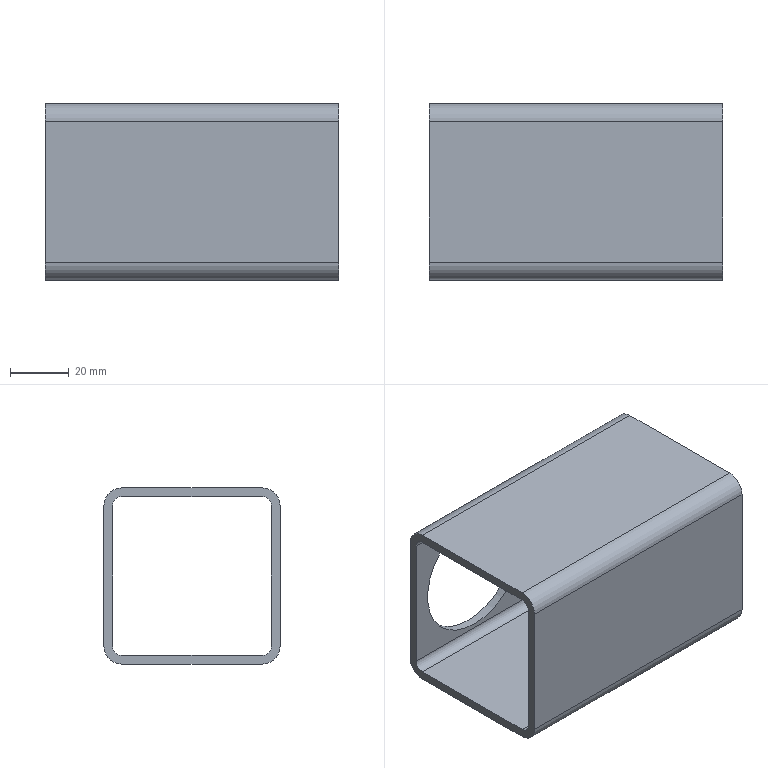Part | STEP file | JBJ-P-1013-03_Default<As Machined> | 1 solid | 19 faces | box 100 x 60 x 60 mm | volume 61311 mm3 | plane 10 | cylinder 9 | commonest cylinder face diameters 6 x4 12 x4 45 x1
STEP:
#1=CARTESIAN_POINT('',(0.,-30.,24.));
#2=VERTEX_POINT('',#1);
#3=CARTESIAN_POINT('',(0.,-24.,30.));
#4=VERTEX_POINT('',#3);
#5=CARTESIAN_POINT('',(0.,-24.,24.));
#6=DIRECTION('',(-1.,0.,0.));
#7=DIRECTION('',(0.,0.,1.));
#8=AXIS2_PLACEMENT_3D('',#5,#6,#7);
#9=CIRCLE('',#8,6.);
#10=EDGE_CURVE('',#2,#4,#9,.T.);
#11=ORIENTED_EDGE('',*,*,#10,.T.);
#12=CARTESIAN_POINT('',(-100.,-24.,30.));
#13=VERTEX_POINT('',#12);
#14=CARTESIAN_POINT('',(-100.,-24.,30.));
#15=DIRECTION('',(1.,0.,0.));
#16=VECTOR('',#15,1000.);
#17=LINE('',#14,#16);
#18=EDGE_CURVE('',#13,#4,#17,.T.);
#19=ORIENTED_EDGE('',*,*,#18,.F.);
#20=CARTESIAN_POINT('',(-100.,-30.,24.));
#21=VERTEX_POINT('',#20);
#22=CARTESIAN_POINT('',(-100.,-24.,24.));
#23=DIRECTION('',(-1.,0.,0.));
#24=DIRECTION('',(0.,0.,1.));
#25=AXIS2_PLACEMENT_3D('',#22,#23,#24);
#26=CIRCLE('',#25,6.);
#27=EDGE_CURVE('',#21,#13,#26,.T.);
#28=ORIENTED_EDGE('',*,*,#27,.F.);
#29=CARTESIAN_POINT('',(-100.,-30.,24.));
#30=DIRECTION('',(1.,0.,0.));
#31=VECTOR('',#30,1000.);
#32=LINE('',#29,#31);
#33=EDGE_CURVE('',#21,#2,#32,.T.);
#34=ORIENTED_EDGE('',*,*,#33,.T.);
#35=EDGE_LOOP('',(#11,#19,#28,#34));
#36=FACE_OUTER_BOUND('',#35,.T.);
#37=CARTESIAN_POINT('',(-100.,-24.,24.));
#38=DIRECTION('',(1.,0.,0.));
#39=DIRECTION('',(0.,0.,-1.));
#40=AXIS2_PLACEMENT_3D('',#37,#38,#39);
#41=CYLINDRICAL_SURFACE('',#40,6.);
#42=ADVANCED_FACE('',(#36),#41,.T.);
#43=CARTESIAN_POINT('',(0.,24.,30.));
#44=VERTEX_POINT('',#43);
#45=CARTESIAN_POINT('',(0.,-24.,30.));
#46=DIRECTION('',(0.,1.,0.));
#47=VECTOR('',#46,1000.);
#48=LINE('',#45,#47);
#49=EDGE_CURVE('',#4,#44,#48,.T.);
#50=ORIENTED_EDGE('',*,*,#49,.T.);
#51=CARTESIAN_POINT('',(-100.,24.,30.));
#52=VERTEX_POINT('',#51);
#53=CARTESIAN_POINT('',(-100.,24.,30.));
#54=DIRECTION('',(1.,0.,0.));
#55=VECTOR('',#54,1000.);
#56=LINE('',#53,#55);
#57=EDGE_CURVE('',#52,#44,#56,.T.);
#58=ORIENTED_EDGE('',*,*,#57,.F.);
#59=CARTESIAN_POINT('',(-100.,-24.,30.));
#60=DIRECTION('',(0.,1.,0.));
#61=VECTOR('',#60,1000.);
#62=LINE('',#59,#61);
#63=EDGE_CURVE('',#13,#52,#62,.T.);
#64=ORIENTED_EDGE('',*,*,#63,.F.);
#65=ORIENTED_EDGE('',*,*,#18,.T.);
#66=EDGE_LOOP('',(#50,#58,#64,#65));
#67=FACE_OUTER_BOUND('',#66,.T.);
#68=CARTESIAN_POINT('',(-100.,-24.,30.));
#69=DIRECTION('',(0.,0.,-1.));
#70=DIRECTION('',(-1.,0.,0.));
#71=AXIS2_PLACEMENT_3D('',#68,#69,#70);
#72=PLANE('',#71);
#73=ADVANCED_FACE('',(#67),#72,.F.);
#74=CARTESIAN_POINT('',(0.,30.,24.));
#75=VERTEX_POINT('',#74);
#76=CARTESIAN_POINT('',(0.,24.,24.));
#77=DIRECTION('',(-1.,0.,0.));
#78=DIRECTION('',(0.,0.,1.));
#79=AXIS2_PLACEMENT_3D('',#76,#77,#78);
#80=CIRCLE('',#79,6.);
#81=EDGE_CURVE('',#44,#75,#80,.T.);
#82=ORIENTED_EDGE('',*,*,#81,.T.);
#83=CARTESIAN_POINT('',(-100.,30.,24.));
#84=VERTEX_POINT('',#83);
#85=CARTESIAN_POINT('',(-100.,30.,24.));
#86=DIRECTION('',(1.,0.,0.));
#87=VECTOR('',#86,1000.);
#88=LINE('',#85,#87);
#89=EDGE_CURVE('',#84,#75,#88,.T.);
#90=ORIENTED_EDGE('',*,*,#89,.F.);
#91=CARTESIAN_POINT('',(-100.,24.,24.));
#92=DIRECTION('',(-1.,0.,0.));
#93=DIRECTION('',(0.,0.,1.));
#94=AXIS2_PLACEMENT_3D('',#91,#92,#93);
#95=CIRCLE('',#94,6.);
#96=EDGE_CURVE('',#52,#84,#95,.T.);
#97=ORIENTED_EDGE('',*,*,#96,.F.);
#98=ORIENTED_EDGE('',*,*,#57,.T.);
#99=EDGE_LOOP('',(#82,#90,#97,#98));
#100=FACE_OUTER_BOUND('',#99,.T.);
#101=CARTESIAN_POINT('',(-100.,24.,24.));
#102=DIRECTION('',(1.,0.,0.));
#103=DIRECTION('',(0.,0.,-1.));
#104=AXIS2_PLACEMENT_3D('',#101,#102,#103);
#105=CYLINDRICAL_SURFACE('',#104,6.);
#106=ADVANCED_FACE('',(#100),#105,.T.);
#107=CARTESIAN_POINT('',(-72.,30.,22.5));
#108=VERTEX_POINT('',#107);
#109=CARTESIAN_POINT('',(-72.,30.,0.));
#110=DIRECTION('',(0.,1.,0.));
#111=DIRECTION('',(0.,0.,1.));
#112=AXIS2_PLACEMENT_3D('',#109,#110,#111);
#113=CIRCLE('',#112,22.5);
#114=EDGE_CURVE('',#108,#108,#113,.T.);
#115=ORIENTED_EDGE('',*,*,#114,.F.);
#116=EDGE_LOOP('',(#115));
#117=FACE_BOUND('',#116,.T.);
#118=CARTESIAN_POINT('',(0.,30.,-24.));
#119=VERTEX_POINT('',#118);
#120=CARTESIAN_POINT('',(0.,30.,-24.));
#121=DIRECTION('',(0.,0.,-1.));
#122=VECTOR('',#121,1000.);
#123=LINE('',#120,#122);
#124=EDGE_CURVE('',#75,#119,#123,.T.);
#125=ORIENTED_EDGE('',*,*,#124,.T.);
#126=CARTESIAN_POINT('',(-100.,30.,-24.));
#127=VERTEX_POINT('',#126);
#128=CARTESIAN_POINT('',(-100.,30.,-24.));
#129=DIRECTION('',(1.,0.,0.));
#130=VECTOR('',#129,1000.);
#131=LINE('',#128,#130);
#132=EDGE_CURVE('',#127,#119,#131,.T.);
#133=ORIENTED_EDGE('',*,*,#132,.F.);
#134=CARTESIAN_POINT('',(-100.,30.,-24.));
#135=DIRECTION('',(0.,0.,-1.));
#136=VECTOR('',#135,1000.);
#137=LINE('',#134,#136);
#138=EDGE_CURVE('',#84,#127,#137,.T.);
#139=ORIENTED_EDGE('',*,*,#138,.F.);
#140=ORIENTED_EDGE('',*,*,#89,.T.);
#141=EDGE_LOOP('',(#125,#133,#139,#140));
#142=FACE_OUTER_BOUND('',#141,.T.);
#143=CARTESIAN_POINT('',(-100.,30.,-24.));
#144=DIRECTION('',(0.,-1.,0.));
#145=DIRECTION('',(0.,0.,-1.));
#146=AXIS2_PLACEMENT_3D('',#143,#144,#145);
#147=PLANE('',#146);
#148=ADVANCED_FACE('',(#117,#142),#147,.F.);
#149=CARTESIAN_POINT('',(0.,24.,-30.));
#150=VERTEX_POINT('',#149);
#151=CARTESIAN_POINT('',(0.,24.,-24.));
#152=DIRECTION('',(-1.,0.,0.));
#153=DIRECTION('',(0.,0.,1.));
#154=AXIS2_PLACEMENT_3D('',#151,#152,#153);
#155=CIRCLE('',#154,6.);
#156=EDGE_CURVE('',#119,#150,#155,.T.);
#157=ORIENTED_EDGE('',*,*,#156,.T.);
#158=CARTESIAN_POINT('',(-100.,24.,-30.));
#159=VERTEX_POINT('',#158);
#160=CARTESIAN_POINT('',(-100.,24.,-30.));
#161=DIRECTION('',(1.,0.,0.));
#162=VECTOR('',#161,1000.);
#163=LINE('',#160,#162);
#164=EDGE_CURVE('',#159,#150,#163,.T.);
#165=ORIENTED_EDGE('',*,*,#164,.F.);
#166=CARTESIAN_POINT('',(-100.,24.,-24.));
#167=DIRECTION('',(-1.,0.,0.));
#168=DIRECTION('',(0.,0.,1.));
#169=AXIS2_PLACEMENT_3D('',#166,#167,#168);
#170=CIRCLE('',#169,6.);
#171=EDGE_CURVE('',#127,#159,#170,.T.);
#172=ORIENTED_EDGE('',*,*,#171,.F.);
#173=ORIENTED_EDGE('',*,*,#132,.T.);
#174=EDGE_LOOP('',(#157,#165,#172,#173));
#175=FACE_OUTER_BOUND('',#174,.T.);
#176=CARTESIAN_POINT('',(-100.,24.,-24.));
#177=DIRECTION('',(1.,0.,0.));
#178=DIRECTION('',(0.,0.,-1.));
#179=AXIS2_PLACEMENT_3D('',#176,#177,#178);
#180=CYLINDRICAL_SURFACE('',#179,6.);
#181=ADVANCED_FACE('',(#175),#180,.T.);
#182=CARTESIAN_POINT('',(0.,-24.,-30.));
#183=VERTEX_POINT('',#182);
#184=CARTESIAN_POINT('',(0.,24.,-30.));
#185=DIRECTION('',(0.,-1.,0.));
#186=VECTOR('',#185,1000.);
#187=LINE('',#184,#186);
#188=EDGE_CURVE('',#150,#183,#187,.T.);
#189=ORIENTED_EDGE('',*,*,#188,.T.);
#190=CARTESIAN_POINT('',(-100.,-24.,-30.));
#191=VERTEX_POINT('',#190);
#192=CARTESIAN_POINT('',(-100.,-24.,-30.));
#193=DIRECTION('',(1.,0.,0.));
#194=VECTOR('',#193,1000.);
#195=LINE('',#192,#194);
#196=EDGE_CURVE('',#191,#183,#195,.T.);
#197=ORIENTED_EDGE('',*,*,#196,.F.);
#198=CARTESIAN_POINT('',(-100.,24.,-30.));
#199=DIRECTION('',(0.,-1.,0.));
#200=VECTOR('',#199,1000.);
#201=LINE('',#198,#200);
#202=EDGE_CURVE('',#159,#191,#201,.T.);
#203=ORIENTED_EDGE('',*,*,#202,.F.);
#204=ORIENTED_EDGE('',*,*,#164,.T.);
#205=EDGE_LOOP('',(#189,#197,#203,#204));
#206=FACE_OUTER_BOUND('',#205,.T.);
#207=CARTESIAN_POINT('',(-100.,24.,-30.));
#208=DIRECTION('',(0.,0.,1.));
#209=DIRECTION('',(1.,0.,0.));
#210=AXIS2_PLACEMENT_3D('',#207,#208,#209);
#211=PLANE('',#210);
#212=ADVANCED_FACE('',(#206),#211,.F.);
#213=CARTESIAN_POINT('',(0.,-30.,-24.));
#214=VERTEX_POINT('',#213);
#215=CARTESIAN_POINT('',(0.,-24.,-24.));
#216=DIRECTION('',(-1.,0.,0.));
#217=DIRECTION('',(0.,0.,1.));
#218=AXIS2_PLACEMENT_3D('',#215,#216,#217);
#219=CIRCLE('',#218,6.);
#220=EDGE_CURVE('',#183,#214,#219,.T.);
#221=ORIENTED_EDGE('',*,*,#220,.T.);
#222=CARTESIAN_POINT('',(-100.,-30.,-24.));
#223=VERTEX_POINT('',#222);
#224=CARTESIAN_POINT('',(-100.,-30.,-24.));
#225=DIRECTION('',(1.,0.,0.));
#226=VECTOR('',#225,1000.);
#227=LINE('',#224,#226);
#228=EDGE_CURVE('',#223,#214,#227,.T.);
#229=ORIENTED_EDGE('',*,*,#228,.F.);
#230=CARTESIAN_POINT('',(-100.,-24.,-24.));
#231=DIRECTION('',(-1.,0.,0.));
#232=DIRECTION('',(0.,0.,1.));
#233=AXIS2_PLACEMENT_3D('',#230,#231,#232);
#234=CIRCLE('',#233,6.);
#235=EDGE_CURVE('',#191,#223,#234,.T.);
#236=ORIENTED_EDGE('',*,*,#235,.F.);
#237=ORIENTED_EDGE('',*,*,#196,.T.);
#238=EDGE_LOOP('',(#221,#229,#236,#237));
#239=FACE_OUTER_BOUND('',#238,.T.);
#240=CARTESIAN_POINT('',(-100.,-24.,-24.));
#241=DIRECTION('',(1.,0.,0.));
#242=DIRECTION('',(0.,0.,-1.));
#243=AXIS2_PLACEMENT_3D('',#240,#241,#242);
#244=CYLINDRICAL_SURFACE('',#243,6.);
#245=ADVANCED_FACE('',(#239),#244,.T.);
#246=CARTESIAN_POINT('',(0.,24.,27.));
#247=VERTEX_POINT('',#246);
#248=CARTESIAN_POINT('',(0.,27.,24.));
#249=VERTEX_POINT('',#248);
#250=CARTESIAN_POINT('',(0.,24.,24.));
#251=DIRECTION('',(-1.,0.,0.));
#252=DIRECTION('',(0.,0.,1.));
#253=AXIS2_PLACEMENT_3D('',#250,#251,#252);
#254=CIRCLE('',#253,3.);
#255=EDGE_CURVE('',#247,#249,#254,.T.);
#256=ORIENTED_EDGE('',*,*,#255,.F.);
#257=CARTESIAN_POINT('',(-100.,24.,27.));
#258=VERTEX_POINT('',#257);
#259=CARTESIAN_POINT('',(-100.,24.,27.));
#260=DIRECTION('',(1.,0.,0.));
#261=VECTOR('',#260,1000.);
#262=LINE('',#259,#261);
#263=EDGE_CURVE('',#258,#247,#262,.T.);
#264=ORIENTED_EDGE('',*,*,#263,.F.);
#265=CARTESIAN_POINT('',(-100.,27.,24.));
#266=VERTEX_POINT('',#265);
#267=CARTESIAN_POINT('',(-100.,24.,24.));
#268=DIRECTION('',(-1.,0.,0.));
#269=DIRECTION('',(0.,0.,1.));
#270=AXIS2_PLACEMENT_3D('',#267,#268,#269);
#271=CIRCLE('',#270,3.);
#272=EDGE_CURVE('',#258,#266,#271,.T.);
#273=ORIENTED_EDGE('',*,*,#272,.T.);
#274=CARTESIAN_POINT('',(-100.,27.,24.));
#275=DIRECTION('',(1.,0.,0.));
#276=VECTOR('',#275,1000.);
#277=LINE('',#274,#276);
#278=EDGE_CURVE('',#266,#249,#277,.T.);
#279=ORIENTED_EDGE('',*,*,#278,.T.);
#280=EDGE_LOOP('',(#256,#264,#273,#279));
#281=FACE_OUTER_BOUND('',#280,.T.);
#282=CARTESIAN_POINT('',(-100.,24.,24.));
#283=DIRECTION('',(1.,0.,0.));
#284=DIRECTION('',(0.,0.,-1.));
#285=AXIS2_PLACEMENT_3D('',#282,#283,#284);
#286=CYLINDRICAL_SURFACE('',#285,3.);
#287=ADVANCED_FACE('',(#281),#286,.F.);
#288=CARTESIAN_POINT('',(0.,-24.,27.));
#289=VERTEX_POINT('',#288);
#290=CARTESIAN_POINT('',(0.,-24.,27.));
#291=DIRECTION('',(0.,1.,0.));
#292=VECTOR('',#291,1000.);
#293=LINE('',#290,#292);
#294=EDGE_CURVE('',#289,#247,#293,.T.);
#295=ORIENTED_EDGE('',*,*,#294,.F.);
#296=CARTESIAN_POINT('',(-100.,-24.,27.));
#297=VERTEX_POINT('',#296);
#298=CARTESIAN_POINT('',(-100.,-24.,27.));
#299=DIRECTION('',(1.,0.,0.));
#300=VECTOR('',#299,1000.);
#301=LINE('',#298,#300);
#302=EDGE_CURVE('',#297,#289,#301,.T.);
#303=ORIENTED_EDGE('',*,*,#302,.F.);
#304=CARTESIAN_POINT('',(-100.,-24.,27.));
#305=DIRECTION('',(0.,1.,0.));
#306=VECTOR('',#305,1000.);
#307=LINE('',#304,#306);
#308=EDGE_CURVE('',#297,#258,#307,.T.);
#309=ORIENTED_EDGE('',*,*,#308,.T.);
#310=ORIENTED_EDGE('',*,*,#263,.T.);
#311=EDGE_LOOP('',(#295,#303,#309,#310));
#312=FACE_OUTER_BOUND('',#311,.T.);
#313=CARTESIAN_POINT('',(-100.,-24.,27.));
#314=DIRECTION('',(0.,0.,-1.));
#315=DIRECTION('',(-1.,0.,0.));
#316=AXIS2_PLACEMENT_3D('',#313,#314,#315);
#317=PLANE('',#316);
#318=ADVANCED_FACE('',(#312),#317,.T.);
#319=CARTESIAN_POINT('',(0.,-27.,24.));
#320=VERTEX_POINT('',#319);
#321=CARTESIAN_POINT('',(0.,-24.,24.));
#322=DIRECTION('',(-1.,0.,0.));
#323=DIRECTION('',(0.,0.,1.));
#324=AXIS2_PLACEMENT_3D('',#321,#322,#323);
#325=CIRCLE('',#324,3.);
#326=EDGE_CURVE('',#320,#289,#325,.T.);
#327=ORIENTED_EDGE('',*,*,#326,.F.);
#328=CARTESIAN_POINT('',(-100.,-27.,24.));
#329=VERTEX_POINT('',#328);
#330=CARTESIAN_POINT('',(-100.,-27.,24.));
#331=DIRECTION('',(1.,0.,0.));
#332=VECTOR('',#331,1000.);
#333=LINE('',#330,#332);
#334=EDGE_CURVE('',#329,#320,#333,.T.);
#335=ORIENTED_EDGE('',*,*,#334,.F.);
#336=CARTESIAN_POINT('',(-100.,-24.,24.));
#337=DIRECTION('',(-1.,0.,0.));
#338=DIRECTION('',(0.,0.,1.));
#339=AXIS2_PLACEMENT_3D('',#336,#337,#338);
#340=CIRCLE('',#339,3.);
#341=EDGE_CURVE('',#329,#297,#340,.T.);
#342=ORIENTED_EDGE('',*,*,#341,.T.);
#343=ORIENTED_EDGE('',*,*,#302,.T.);
#344=EDGE_LOOP('',(#327,#335,#342,#343));
#345=FACE_OUTER_BOUND('',#344,.T.);
#346=CARTESIAN_POINT('',(-100.,-24.,24.));
#347=DIRECTION('',(1.,0.,0.));
#348=DIRECTION('',(0.,0.,-1.));
#349=AXIS2_PLACEMENT_3D('',#346,#347,#348);
#350=CYLINDRICAL_SURFACE('',#349,3.);
#351=ADVANCED_FACE('',(#345),#350,.F.);
#352=CARTESIAN_POINT('',(0.,-27.,-24.));
#353=VERTEX_POINT('',#352);
#354=CARTESIAN_POINT('',(0.,-27.,24.));
#355=DIRECTION('',(0.,0.,1.));
#356=VECTOR('',#355,1000.);
#357=LINE('',#354,#356);
#358=EDGE_CURVE('',#353,#320,#357,.T.);
#359=ORIENTED_EDGE('',*,*,#358,.F.);
#360=CARTESIAN_POINT('',(-100.,-27.,-24.));
#361=VERTEX_POINT('',#360);
#362=CARTESIAN_POINT('',(-100.,-27.,-24.));
#363=DIRECTION('',(1.,0.,0.));
#364=VECTOR('',#363,1000.);
#365=LINE('',#362,#364);
#366=EDGE_CURVE('',#361,#353,#365,.T.);
#367=ORIENTED_EDGE('',*,*,#366,.F.);
#368=CARTESIAN_POINT('',(-100.,-27.,24.));
#369=DIRECTION('',(0.,0.,1.));
#370=VECTOR('',#369,1000.);
#371=LINE('',#368,#370);
#372=EDGE_CURVE('',#361,#329,#371,.T.);
#373=ORIENTED_EDGE('',*,*,#372,.T.);
#374=ORIENTED_EDGE('',*,*,#334,.T.);
#375=EDGE_LOOP('',(#359,#367,#373,#374));
#376=FACE_OUTER_BOUND('',#375,.T.);
#377=CARTESIAN_POINT('',(-100.,-27.,24.));
#378=DIRECTION('',(0.,1.,0.));
#379=DIRECTION('',(0.,0.,1.));
#380=AXIS2_PLACEMENT_3D('',#377,#378,#379);
#381=PLANE('',#380);
#382=ADVANCED_FACE('',(#376),#381,.T.);
#383=CARTESIAN_POINT('',(0.,-24.,-27.));
#384=VERTEX_POINT('',#383);
#385=CARTESIAN_POINT('',(0.,-24.,-24.));
#386=DIRECTION('',(-1.,0.,0.));
#387=DIRECTION('',(0.,0.,1.));
#388=AXIS2_PLACEMENT_3D('',#385,#386,#387);
#389=CIRCLE('',#388,3.);
#390=EDGE_CURVE('',#384,#353,#389,.T.);
#391=ORIENTED_EDGE('',*,*,#390,.F.);
#392=CARTESIAN_POINT('',(-100.,-24.,-27.));
#393=VERTEX_POINT('',#392);
#394=CARTESIAN_POINT('',(-100.,-24.,-27.));
#395=DIRECTION('',(1.,0.,0.));
#396=VECTOR('',#395,1000.);
#397=LINE('',#394,#396);
#398=EDGE_CURVE('',#393,#384,#397,.T.);
#399=ORIENTED_EDGE('',*,*,#398,.F.);
#400=CARTESIAN_POINT('',(-100.,-24.,-24.));
#401=DIRECTION('',(-1.,0.,0.));
#402=DIRECTION('',(0.,0.,1.));
#403=AXIS2_PLACEMENT_3D('',#400,#401,#402);
#404=CIRCLE('',#403,3.);
#405=EDGE_CURVE('',#393,#361,#404,.T.);
#406=ORIENTED_EDGE('',*,*,#405,.T.);
#407=ORIENTED_EDGE('',*,*,#366,.T.);
#408=EDGE_LOOP('',(#391,#399,#406,#407));
#409=FACE_OUTER_BOUND('',#408,.T.);
#410=CARTESIAN_POINT('',(-100.,-24.,-24.));
#411=DIRECTION('',(1.,0.,0.));
#412=DIRECTION('',(0.,0.,-1.));
#413=AXIS2_PLACEMENT_3D('',#410,#411,#412);
#414=CYLINDRICAL_SURFACE('',#413,3.);
#415=ADVANCED_FACE('',(#409),#414,.F.);
#416=CARTESIAN_POINT('',(0.,24.,-27.));
#417=VERTEX_POINT('',#416);
#418=CARTESIAN_POINT('',(0.,24.,-27.));
#419=DIRECTION('',(0.,-1.,0.));
#420=VECTOR('',#419,1000.);
#421=LINE('',#418,#420);
#422=EDGE_CURVE('',#417,#384,#421,.T.);
#423=ORIENTED_EDGE('',*,*,#422,.F.);
#424=CARTESIAN_POINT('',(-100.,24.,-27.));
#425=VERTEX_POINT('',#424);
#426=CARTESIAN_POINT('',(-100.,24.,-27.));
#427=DIRECTION('',(1.,0.,0.));
#428=VECTOR('',#427,1000.);
#429=LINE('',#426,#428);
#430=EDGE_CURVE('',#425,#417,#429,.T.);
#431=ORIENTED_EDGE('',*,*,#430,.F.);
#432=CARTESIAN_POINT('',(-100.,24.,-27.));
#433=DIRECTION('',(0.,-1.,0.));
#434=VECTOR('',#433,1000.);
#435=LINE('',#432,#434);
#436=EDGE_CURVE('',#425,#393,#435,.T.);
#437=ORIENTED_EDGE('',*,*,#436,.T.);
#438=ORIENTED_EDGE('',*,*,#398,.T.);
#439=EDGE_LOOP('',(#423,#431,#437,#438));
#440=FACE_OUTER_BOUND('',#439,.T.);
#441=CARTESIAN_POINT('',(-100.,24.,-27.));
#442=DIRECTION('',(0.,0.,1.));
#443=DIRECTION('',(1.,0.,0.));
#444=AXIS2_PLACEMENT_3D('',#441,#442,#443);
#445=PLANE('',#444);
#446=ADVANCED_FACE('',(#440),#445,.T.);
#447=CARTESIAN_POINT('',(0.,27.,-24.));
#448=VERTEX_POINT('',#447);
#449=CARTESIAN_POINT('',(0.,24.,-24.));
#450=DIRECTION('',(-1.,0.,0.));
#451=DIRECTION('',(0.,0.,1.));
#452=AXIS2_PLACEMENT_3D('',#449,#450,#451);
#453=CIRCLE('',#452,3.);
#454=EDGE_CURVE('',#448,#417,#453,.T.);
#455=ORIENTED_EDGE('',*,*,#454,.F.);
#456=CARTESIAN_POINT('',(-100.,27.,-24.));
#457=VERTEX_POINT('',#456);
#458=CARTESIAN_POINT('',(-100.,27.,-24.));
#459=DIRECTION('',(1.,0.,0.));
#460=VECTOR('',#459,1000.);
#461=LINE('',#458,#460);
#462=EDGE_CURVE('',#457,#448,#461,.T.);
#463=ORIENTED_EDGE('',*,*,#462,.F.);
#464=CARTESIAN_POINT('',(-100.,24.,-24.));
#465=DIRECTION('',(-1.,0.,0.));
#466=DIRECTION('',(0.,0.,1.));
#467=AXIS2_PLACEMENT_3D('',#464,#465,#466);
#468=CIRCLE('',#467,3.);
#469=EDGE_CURVE('',#457,#425,#468,.T.);
#470=ORIENTED_EDGE('',*,*,#469,.T.);
#471=ORIENTED_EDGE('',*,*,#430,.T.);
#472=EDGE_LOOP('',(#455,#463,#470,#471));
#473=FACE_OUTER_BOUND('',#472,.T.);
#474=CARTESIAN_POINT('',(-100.,24.,-24.));
#475=DIRECTION('',(1.,0.,0.));
#476=DIRECTION('',(0.,0.,-1.));
#477=AXIS2_PLACEMENT_3D('',#474,#475,#476);
#478=CYLINDRICAL_SURFACE('',#477,3.);
#479=ADVANCED_FACE('',(#473),#478,.F.);
#480=CARTESIAN_POINT('',(-72.,27.,-22.5));
#481=VERTEX_POINT('',#480);
#482=CARTESIAN_POINT('',(-72.,27.,0.));
#483=DIRECTION('',(0.,1.,0.));
#484=DIRECTION('',(0.,0.,-1.));
#485=AXIS2_PLACEMENT_3D('',#482,#483,#484);
#486=CIRCLE('',#485,22.5);
#487=EDGE_CURVE('',#481,#481,#486,.T.);
#488=ORIENTED_EDGE('',*,*,#487,.T.);
#489=EDGE_LOOP('',(#488));
#490=FACE_BOUND('',#489,.T.);
#491=CARTESIAN_POINT('',(0.,27.,-24.));
#492=DIRECTION('',(0.,0.,-1.));
#493=VECTOR('',#492,1000.);
#494=LINE('',#491,#493);
#495=EDGE_CURVE('',#249,#448,#494,.T.);
#496=ORIENTED_EDGE('',*,*,#495,.F.);
#497=ORIENTED_EDGE('',*,*,#278,.F.);
#498=CARTESIAN_POINT('',(-100.,27.,-24.));
#499=DIRECTION('',(0.,0.,-1.));
#500=VECTOR('',#499,1000.);
#501=LINE('',#498,#500);
#502=EDGE_CURVE('',#266,#457,#501,.T.);
#503=ORIENTED_EDGE('',*,*,#502,.T.);
#504=ORIENTED_EDGE('',*,*,#462,.T.);
#505=EDGE_LOOP('',(#496,#497,#503,#504));
#506=FACE_OUTER_BOUND('',#505,.T.);
#507=CARTESIAN_POINT('',(-100.,27.,-24.));
#508=DIRECTION('',(0.,-1.,0.));
#509=DIRECTION('',(0.,0.,-1.));
#510=AXIS2_PLACEMENT_3D('',#507,#508,#509);
#511=PLANE('',#510);
#512=ADVANCED_FACE('',(#490,#506),#511,.T.);
#513=CARTESIAN_POINT('',(0.,-30.,24.));
#514=DIRECTION('',(0.,0.,1.));
#515=VECTOR('',#514,1000.);
#516=LINE('',#513,#515);
#517=EDGE_CURVE('',#214,#2,#516,.T.);
#518=ORIENTED_EDGE('',*,*,#517,.T.);
#519=ORIENTED_EDGE('',*,*,#33,.F.);
#520=CARTESIAN_POINT('',(-100.,-30.,24.));
#521=DIRECTION('',(0.,0.,1.));
#522=VECTOR('',#521,1000.);
#523=LINE('',#520,#522);
#524=EDGE_CURVE('',#223,#21,#523,.T.);
#525=ORIENTED_EDGE('',*,*,#524,.F.);
#526=ORIENTED_EDGE('',*,*,#228,.T.);
#527=EDGE_LOOP('',(#518,#519,#525,#526));
#528=FACE_OUTER_BOUND('',#527,.T.);
#529=CARTESIAN_POINT('',(-100.,-30.,24.));
#530=DIRECTION('',(0.,1.,0.));
#531=DIRECTION('',(0.,0.,1.));
#532=AXIS2_PLACEMENT_3D('',#529,#530,#531);
#533=PLANE('',#532);
#534=ADVANCED_FACE('',(#528),#533,.F.);
#535=ORIENTED_EDGE('',*,*,#272,.F.);
#536=ORIENTED_EDGE('',*,*,#308,.F.);
#537=ORIENTED_EDGE('',*,*,#341,.F.);
#538=ORIENTED_EDGE('',*,*,#372,.F.);
#539=ORIENTED_EDGE('',*,*,#405,.F.);
#540=ORIENTED_EDGE('',*,*,#436,.F.);
#541=ORIENTED_EDGE('',*,*,#469,.F.);
#542=ORIENTED_EDGE('',*,*,#502,.F.);
#543=EDGE_LOOP('',(#535,#536,#537,#538,#539,#540,#541,#542));
#544=FACE_BOUND('',#543,.T.);
#545=ORIENTED_EDGE('',*,*,#27,.T.);
#546=ORIENTED_EDGE('',*,*,#63,.T.);
#547=ORIENTED_EDGE('',*,*,#96,.T.);
#548=ORIENTED_EDGE('',*,*,#138,.T.);
#549=ORIENTED_EDGE('',*,*,#171,.T.);
#550=ORIENTED_EDGE('',*,*,#202,.T.);
#551=ORIENTED_EDGE('',*,*,#235,.T.);
#552=ORIENTED_EDGE('',*,*,#524,.T.);
#553=EDGE_LOOP('',(#545,#546,#547,#548,#549,#550,#551,#552));
#554=FACE_OUTER_BOUND('',#553,.T.);
#555=CARTESIAN_POINT('',(-100.,-24.,24.));
#556=DIRECTION('',(-1.,0.,0.));
#557=DIRECTION('',(0.,0.,1.));
#558=AXIS2_PLACEMENT_3D('',#555,#556,#557);
#559=PLANE('',#558);
#560=ADVANCED_FACE('',(#544,#554),#559,.T.);
#561=ORIENTED_EDGE('',*,*,#255,.T.);
#562=ORIENTED_EDGE('',*,*,#495,.T.);
#563=ORIENTED_EDGE('',*,*,#454,.T.);
#564=ORIENTED_EDGE('',*,*,#422,.T.);
#565=ORIENTED_EDGE('',*,*,#390,.T.);
#566=ORIENTED_EDGE('',*,*,#358,.T.);
#567=ORIENTED_EDGE('',*,*,#326,.T.);
#568=ORIENTED_EDGE('',*,*,#294,.T.);
#569=EDGE_LOOP('',(#561,#562,#563,#564,#565,#566,#567,#568));
#570=FACE_BOUND('',#569,.T.);
#571=ORIENTED_EDGE('',*,*,#10,.F.);
#572=ORIENTED_EDGE('',*,*,#517,.F.);
#573=ORIENTED_EDGE('',*,*,#220,.F.);
#574=ORIENTED_EDGE('',*,*,#188,.F.);
#575=ORIENTED_EDGE('',*,*,#156,.F.);
#576=ORIENTED_EDGE('',*,*,#124,.F.);
#577=ORIENTED_EDGE('',*,*,#81,.F.);
#578=ORIENTED_EDGE('',*,*,#49,.F.);
#579=EDGE_LOOP('',(#571,#572,#573,#574,#575,#576,#577,#578));
#580=FACE_OUTER_BOUND('',#579,.T.);
#581=CARTESIAN_POINT('',(0.,-24.,24.));
#582=DIRECTION('',(-1.,0.,0.));
#583=DIRECTION('',(0.,0.,1.));
#584=AXIS2_PLACEMENT_3D('',#581,#582,#583);
#585=PLANE('',#584);
#586=ADVANCED_FACE('',(#570,#580),#585,.F.);
#587=ORIENTED_EDGE('',*,*,#487,.F.);
#588=EDGE_LOOP('',(#587));
#589=FACE_OUTER_BOUND('',#588,.T.);
#590=ORIENTED_EDGE('',*,*,#114,.T.);
#591=EDGE_LOOP('',(#590));
#592=FACE_OUTER_BOUND('',#591,.T.);
#593=CARTESIAN_POINT('',(-72.,-30.001,0.));
#594=DIRECTION('',(0.,1.,0.));
#595=DIRECTION('',(0.,0.,1.));
#596=AXIS2_PLACEMENT_3D('',#593,#594,#595);
#597=CYLINDRICAL_SURFACE('',#596,22.5);
#598=ADVANCED_FACE('',(#589,#592),#597,.F.);
#599=CLOSED_SHELL('',(#42,#73,#106,#148,#181,#212,#245,#287,#318,#351,#382,#415,#446,#479,#512,#534,#560,#586,#598));
#600=MANIFOLD_SOLID_BREP('',#599);
#601=CARTESIAN_POINT('',(0.,0.,0.));
#602=DIRECTION('',(0.,0.,1.));
#603=DIRECTION('',(1.,0.,0.));
#604=AXIS2_PLACEMENT_3D('',#601,#602,#603);
#605=(LENGTH_UNIT()NAMED_UNIT(*)SI_UNIT(.MILLI.,.METRE.));
#606=UNCERTAINTY_MEASURE_WITH_UNIT(LENGTH_MEASURE(0.00001),#605,'','');
#607=(NAMED_UNIT(*)PLANE_ANGLE_UNIT()SI_UNIT($,.RADIAN.));
#608=(NAMED_UNIT(*)SI_UNIT($,.STERADIAN.)SOLID_ANGLE_UNIT());
#609=(GEOMETRIC_REPRESENTATION_CONTEXT(3)GLOBAL_UNCERTAINTY_ASSIGNED_CONTEXT((#606))GLOBAL_UNIT_ASSIGNED_CONTEXT((#605,#607,#608))REPRESENTATION_CONTEXT('',''));
#610=ADVANCED_BREP_SHAPE_REPRESENTATION('',(#600,#604),#609);